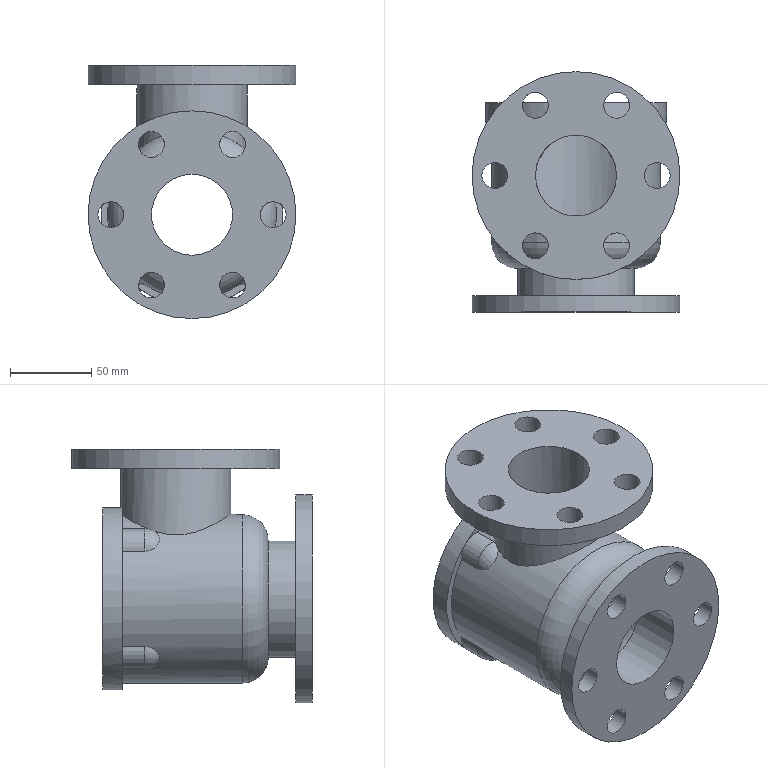Part | NX | features EXTRUDE 6, DATUM_CSYS 5, SIMPLE HOLE 4, SKETCH 4, SYMBOLIC_THREAD 4, BLEND 1, HOLE PACKAGE 1, REPLACE_FACE 1, SWP104 1, UNITE 1 | 1 solid | 72 faces | box 128 x 148 x 156 mm | volume 660287 mm3 | cylinder 38 | plane 16 | sphere 8 | cone 8 | torus 2 | commonest cylinder face diameters 16 x12 24 x8 10.3 x4 104 x3 50 x2 72 x2